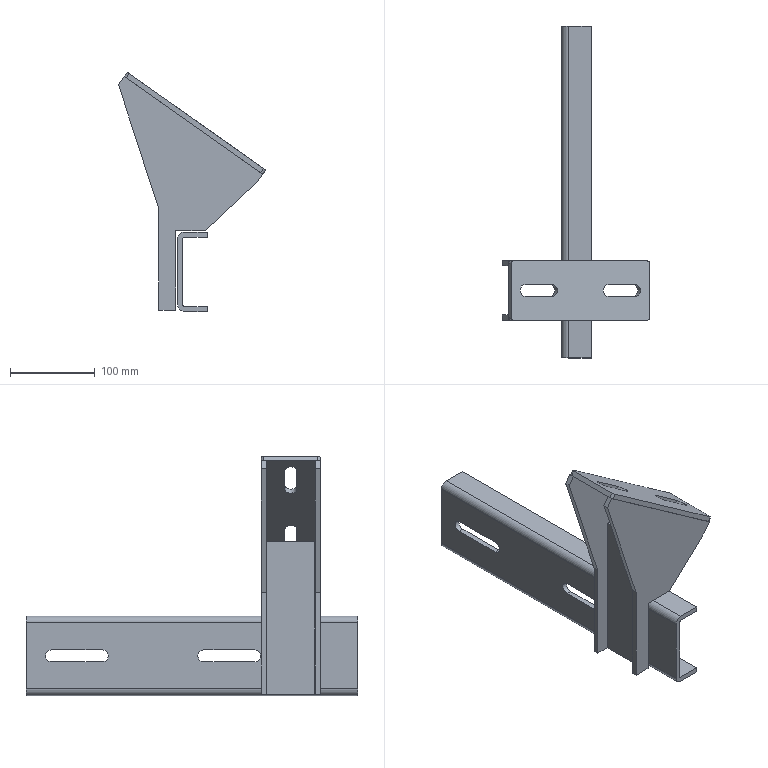Part | STEP file | HL4GZ-1.30.036 (left cane-feed front mounting seat weldment) | 5 solids | 68 faces | box 173.767 x 392 x 282.649 mm | volume 650486 mm3 | plane 52 | cylinder 16 | commonest cylinder face diameters 14 x8 6 x4 4 x2 16 x2